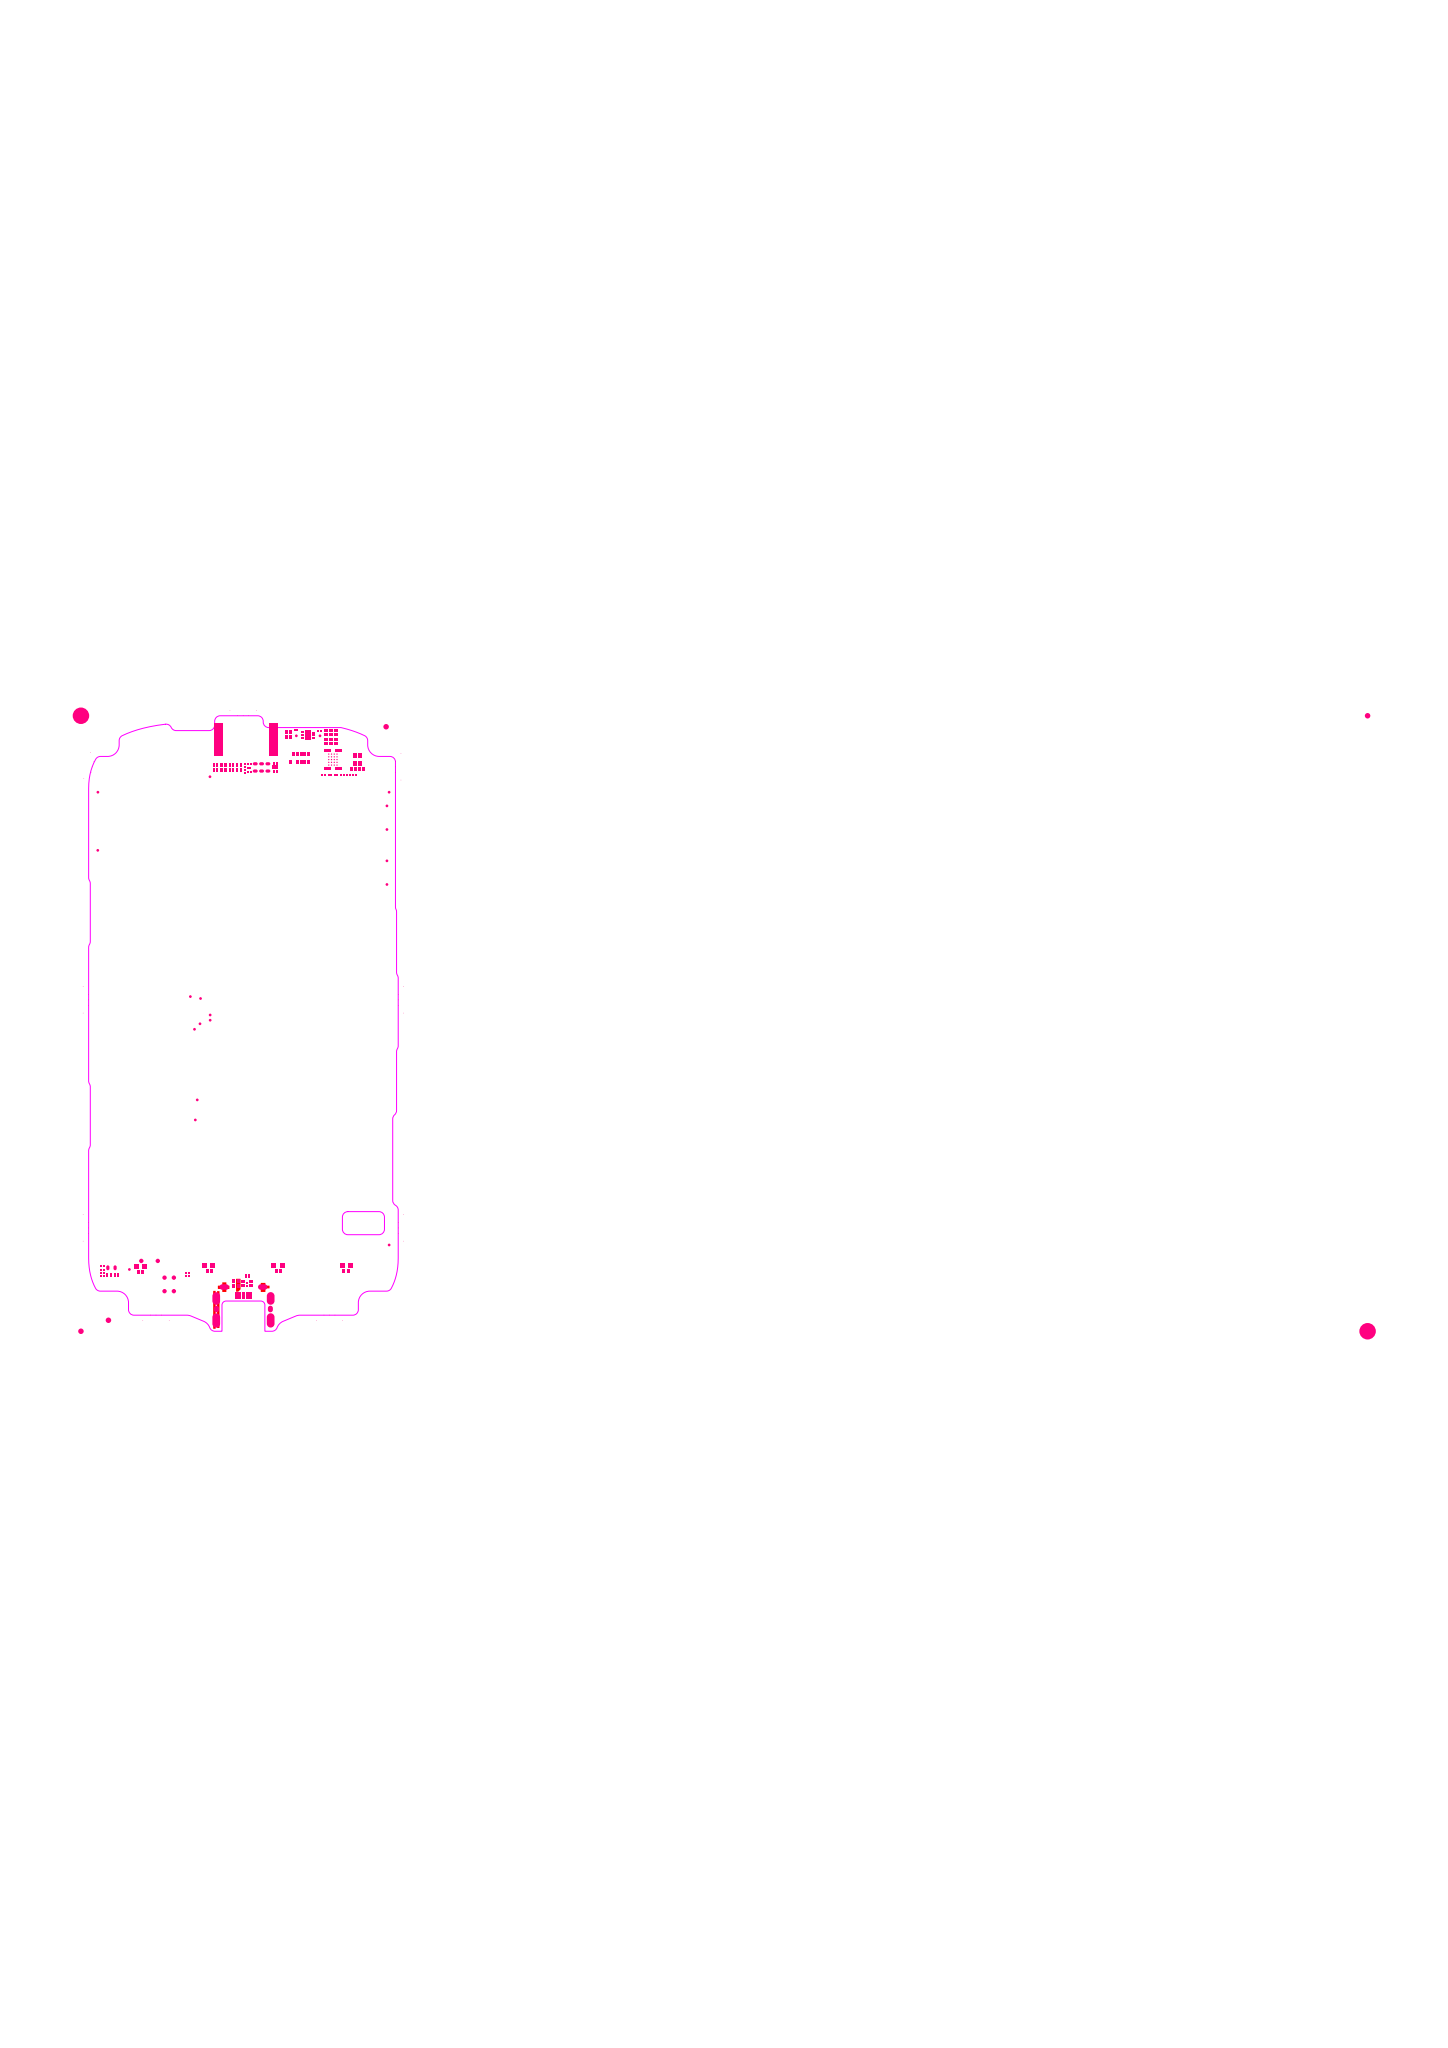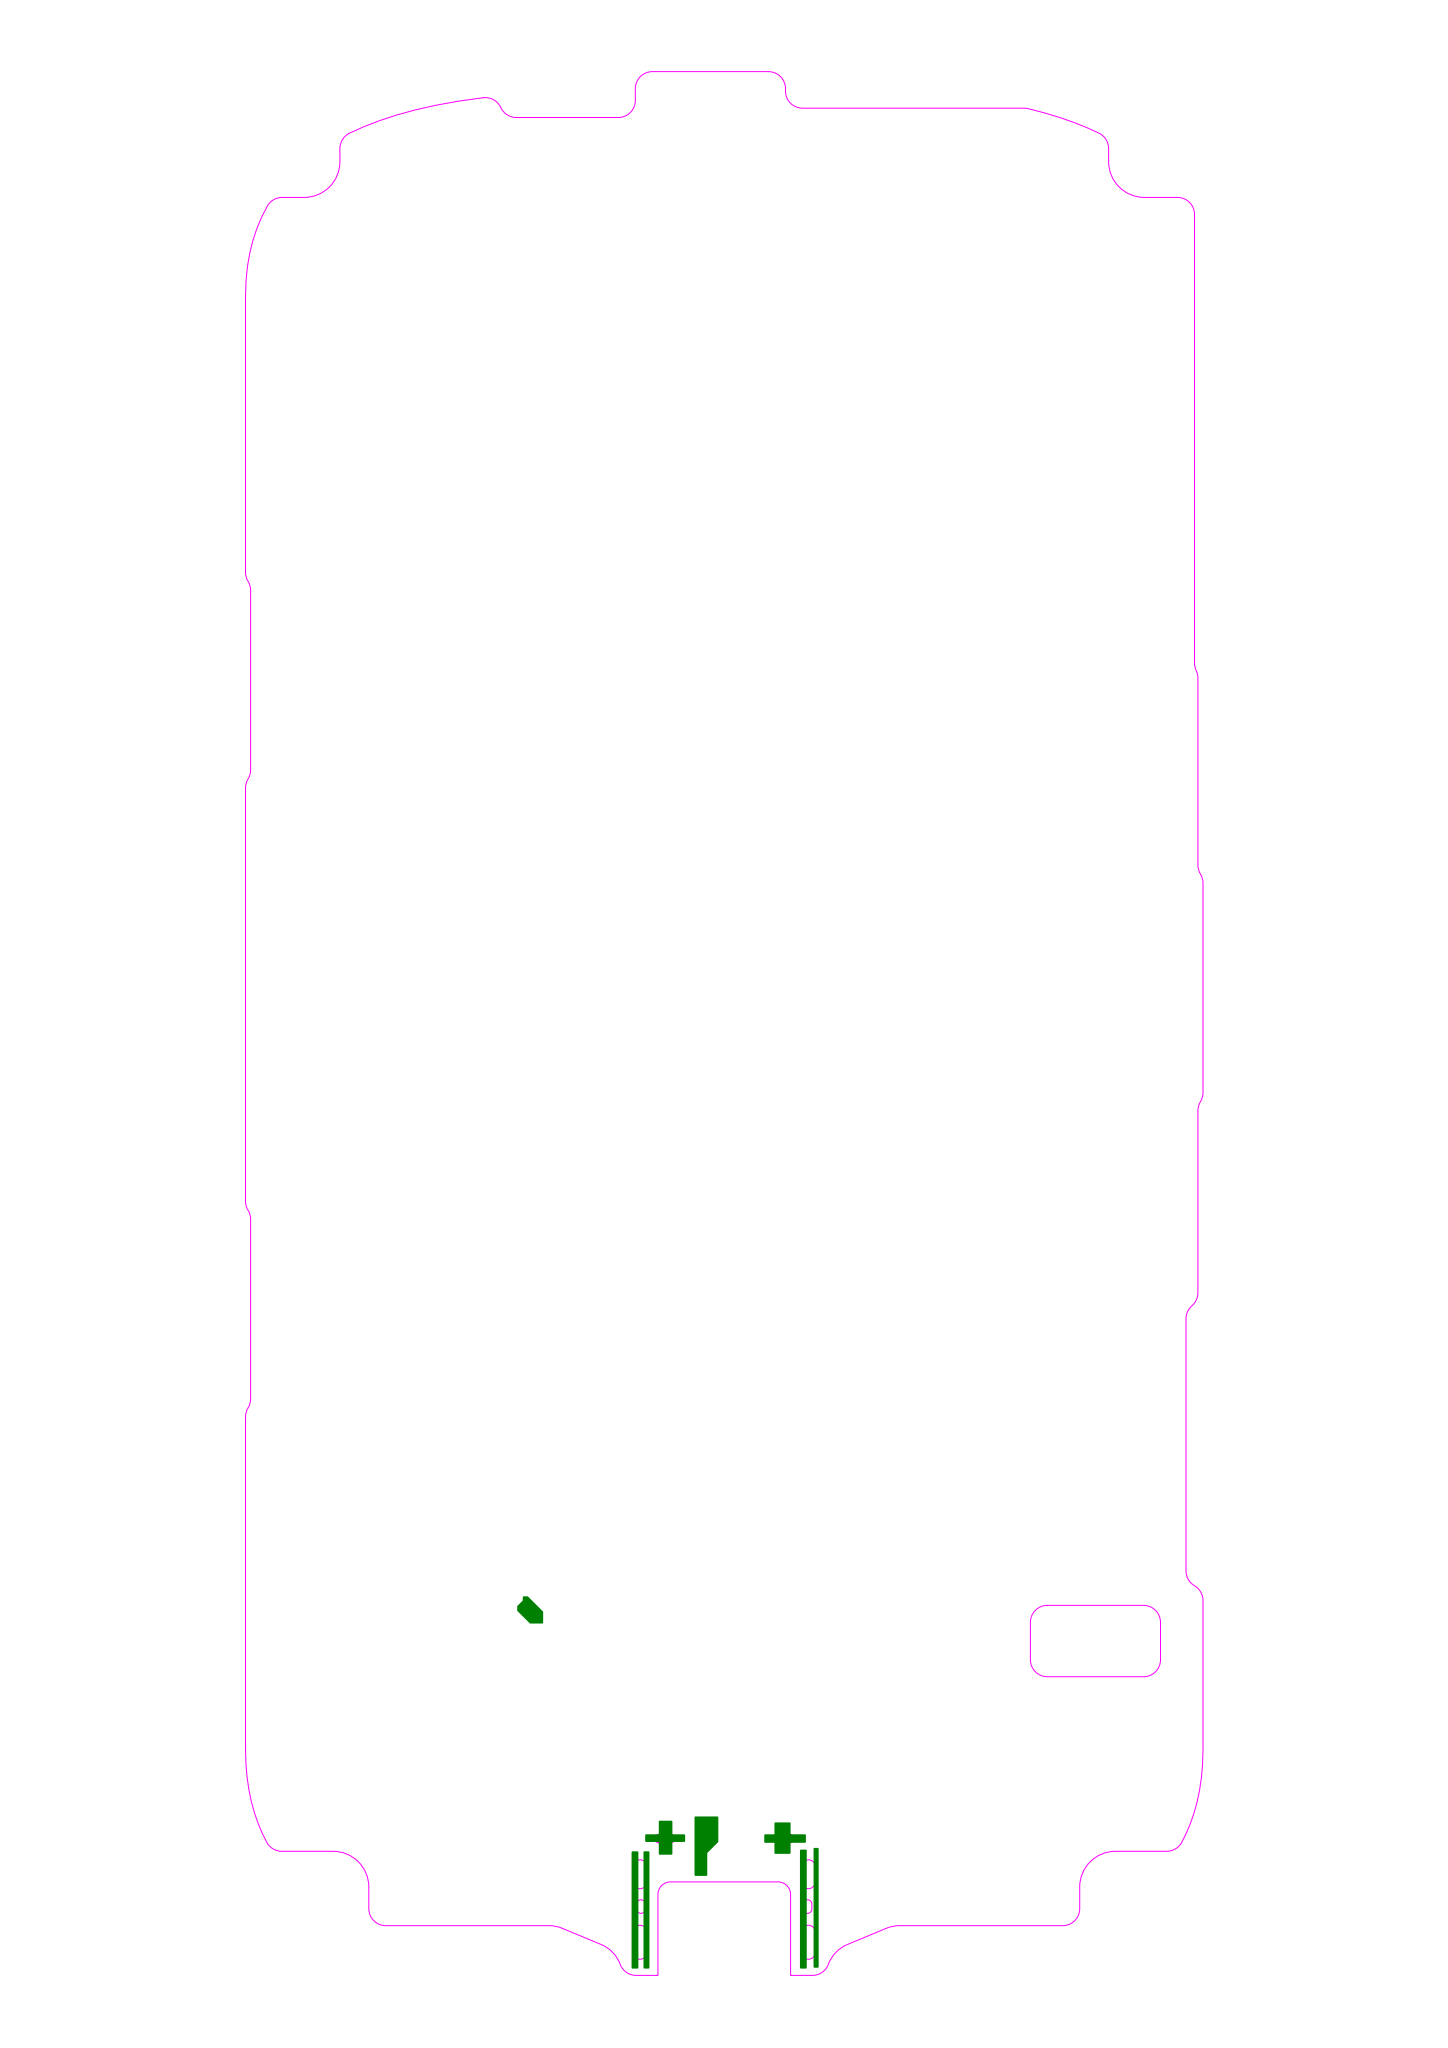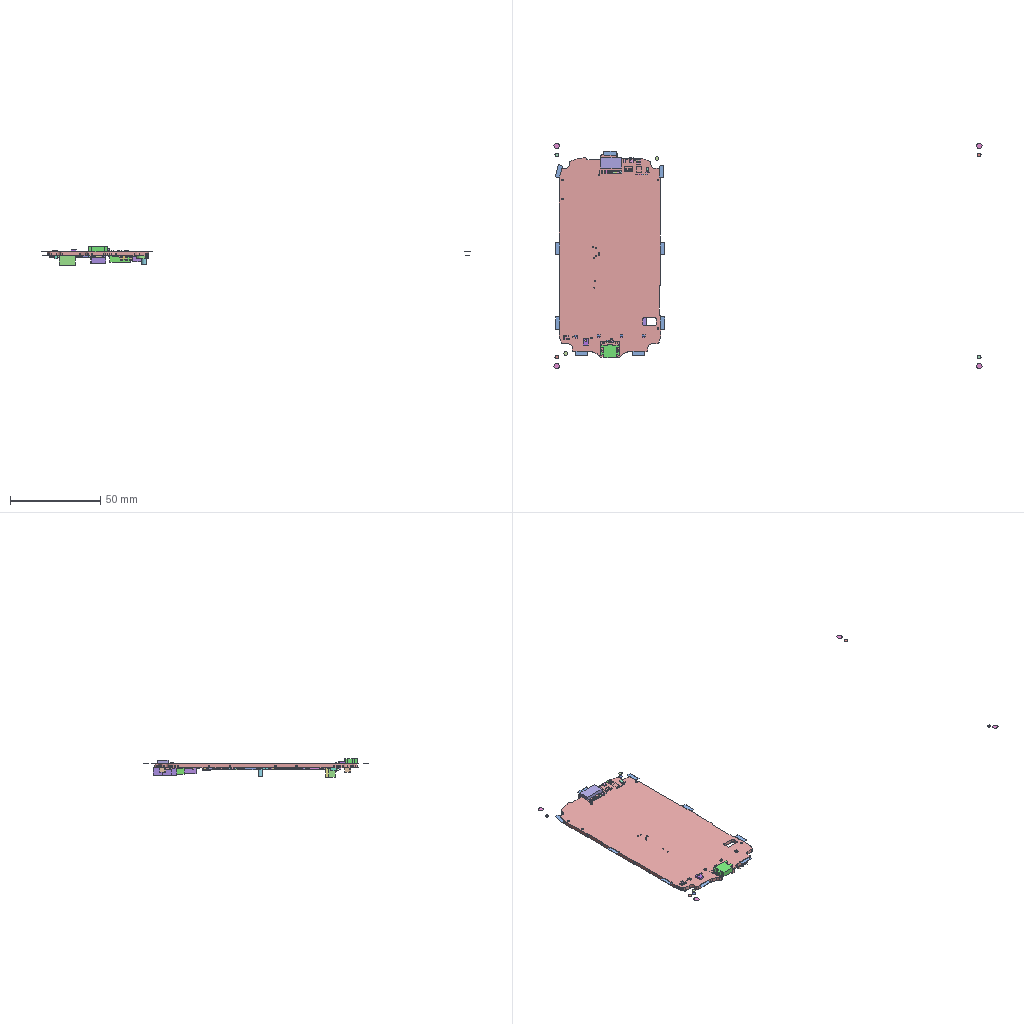Circuit board layout | Siemens PADS | box 237 x 125 x 10.3 mm
Layer stack:
layer,name,type,plane,layer_thickness_mm,copper_thickness_mm,dielectric_constant
0,,,,0,,3.3
1,Top,ROUTING,NONE,0.254,0.03429,4.3
2,Inner Layer 2,ROUTING,NONE,0.254,0.03429,4.3
3,Inner Layer 3,ROUTING,NONE,0.254,0.03429,4.3
4,Inner Layer 4,ROUTING,NONE,0.254,0.03429,4.3
5,Inner Layer 5,ROUTING,NONE,0.254,0.03429,4.3
6,Inner Layer 6,ROUTING,NONE,0.254,0.03429,4.3
7,Inner Layer 7,ROUTING,NONE,0.254,0.03429,4.3
8,Bottom,ROUTING,NONE,0,0.03429,3.3
Part placement, first 418 of 814 lines:
Ref,PartType,Decal,X_mm,Y_mm,Rotation,Layer,Placed,Installed
ANT_GPS1,HT11.011.30120,HT11.011.30120,50.55,117.8,90,Bottom,True,True
ANT_GPS2,HT11.011.30120,HT11.011.30120,53.25,117.8,90,Bottom,True,True
ANT_MAIN1,HT11.011.30120,HT11.011.30120,50.075,15.825,90,Bottom,True,True
ANT_MAIN2,HT11.011.30120,HT11.011.30120,52.775,15.825,90,Bottom,True,True
ANT_MAIN3,HT11.011.30120,HT11.011.30120,47.375,15.825,90,Bottom,True,True
ANT_WLAN1,HT11.011.30120,HT11.011.30120,18.056,118.25,90,Bottom,True,True
ANT_WLAN2,HT11.011.30120,HT11.011.30120,15.35,118.25,90,Bottom,False,True
B201,4700043A001,GZ1005,25.5,60.6,0,Bottom,True,True
B501,4700043A001,GZ1005,25.65,93.05,90,Bottom,True,True
B502,4700043A001,GZ1005,25.65,94.55,90,Bottom,True,True
B503,4700043A001,GZ1005,11.65,103.5,0,Bottom,True,True
B504,4700043A001,GZ1005,11.7,102.45,0,Bottom,True,True
B505,2400006A033,IND0402_0.55,30.9,112.15,180,Top,True,True
B506,2400006A033,IND0402_0.55,30.9,113.1,180,Top,True,True
B507,4700043A001,GZ1005,40.69,114.32,90,Bottom,True,True
B508,4700050A001,GZ1005,41.04,117.62,0,Bottom,True,True
B601,4700039A001,PZ2012U,12.75,29.2,0,Bottom,True,True
B701,4700039A001,PZ2012U,32.5,27.1,270,Bottom,True,True
B901,4700043A001,GZ1005,13,69.05,180,Bottom,True,True
B1001,4700043A001,GZ1005,22,109.9,0,Bottom,True,True
B1101,4700043A001,GZ1005,49.5,118.9,270,Top,True,True
BAT301,KS414F-ER,KS414F-ER,58.15,22.8,90,Bottom,True,True
BREAK1,BREAKAWAY_3,BREAKAWAY_3,6.4,28.8,90,Top,False,True
BREAK2,BREAKAWAY_3,BREAKAWAY_3,18.65,12.95,180,Top,False,True
BREAK3,BREAKAWAY_3,BREAKAWAY_3,50.2,12.95,180,Top,False,True
BREAK5,BREAKAWAY_3,BREAKAWAY_3,34.5,122,0,Top,False,True
BREAK7,BREAKAWAY_3,BREAKAWAY_3,62.7,70.3,270,Top,False,True
BREAK8,BREAKAWAY_3,BREAKAWAY_3,7.1,112.7,75.343,Top,False,True
BREAK9,BREAKAWAY_3,BREAKAWAY_3,6.4,70.3,90,Top,False,True
BREAK10,BREAKAWAY_3,BREAKAWAY_3,62.2,112.7,270,Top,False,True
BREAK11,BREAKAWAY_3,BREAKAWAY_3,62.7,28.8,270,Top,False,True
C101,2100011A026,CAP0603_0.95,34.05,70.95,270,Bottom,True,True
C102,2100015A028,CAP0805_0.95,29.45,60.1,0,Bottom,True,True
C103,2100002A032,CAP0201_0.33,34.4,73.5,270,Bottom,True,True
C104,2100002A021,CAP0201_0.33,20.7,72.9,270,Bottom,True,True
C105,2100002A032,CAP0201_0.33,29.3,61.5,0,Bottom,True,True
C106,2100002A021,CAP0201_0.33,18.1,62.35,270,Bottom,True,True
C107,2100002A032,CAP0201_0.33,20.65,75.15,0,Bottom,True,True
C108,2100002A021_DNP,CAP0201_0.33_DNP,29.3,62.7,0,Bottom,True,True
C109,2100002A032_DNP,CAP0201_0.33_DNP,18.7,62.35,270,Bottom,True,True
C110,2100002A021_DNP,CAP0201_0.33_DNP,18.3,63.45,90,Bottom,True,True
C111,2100002A032_DNP,CAP0201_0.33_DNP,19.9,62.35,270,Bottom,True,True
C112,2100002A021_DNP,CAP0201_0.33_DNP,18.95,63.45,90,Bottom,True,True
C113,2100002A032_DNP,CAP0201_0.33_DNP,20.65,75.75,0,Bottom,True,True
C114,2100002A032,CAP0201_0.33,33.8,73.5,270,Bottom,True,True
C115,2100002A032,CAP0201_0.33,19.6,63.45,90,Bottom,True,True
C116,2100002A032,CAP0201_0.33,20.65,73.95,0,Bottom,True,True
C117,2100002A032,CAP0201_0.33,29.3,62.1,0,Bottom,True,True
C118,2100002A032,CAP0201_0.33,19.3,62.35,270,Bottom,True,True
C119,2100002A032,CAP0201_0.33,35,73,270,Bottom,True,True
C122,2100002A032_DNP,CAP0201_0.33_DNP,20.65,74.55,0,Bottom,True,True
C126,2100015A028,CAP0805_0.95,19.55,64.85,0,Bottom,True,True
C127,2100002A021,CAP0201_0.33,20.5,65.95,180,Bottom,True,True
C128,2100002A032,CAP0201_0.33,19.6,66.2,90,Bottom,True,True
C129,2100002A032_DNP,CAP0201_0.33_DNP,19,66.2,90,Bottom,True,True
C130,2100011A026,CAP0603_0.95,33.3,76.55,90,Bottom,True,True
C131,2100002A021,CAP0201_0.33,33.975,74.95,0,Bottom,True,True
C132,2100002A032,CAP0201_0.33,34.95,81.5,90,Bottom,True,True
C134,2100002A032,CAP0201_0.33,34.95,80.4,270,Bottom,True,True
C137,2100002A032,CAP0201_0.33,34.95,79.3,90,Bottom,True,True
C138,2100002A038,CAP0201_0.33,34.95,78.2,270,Bottom,True,True
C140,2100011A026,CAP0603_0.95,17.4,64.75,270,Bottom,True,True
C141,2100002A038,CAP0201_0.33,18.1,67.4,0,Bottom,True,True
C142,2100002A032,CAP0201_0.33,19,67.3,270,Bottom,True,True
C143,2100002A038,CAP0201_0.33,18.1,66.15,0,Bottom,True,True
C144,2100002A032_DNP,CAP0201_0.33_DNP,19.6,67.3,270,Bottom,True,True
C145,2100002A032_DNP,CAP0201_0.33_DNP,20.2,67.3,270,Bottom,True,True
C146,2100002A032_DNP,CAP0201_0.33_DNP,18.1,66.75,0,Bottom,True,True
C147,2100002A038,CAP0201_0.33,25.65,59.6,270,Bottom,True,True
C148,2100002A038,CAP0201_0.33,26.55,60.6,270,Bottom,True,True
C149,2100002A038,CAP0201_0.33,23.5,61.55,0,Bottom,True,True
C150,2100006A034,CAP0402_0.55,19.9,70.9,0,Bottom,True,True
C151,2100002A038,CAP0201_0.33,20.1,71.7,0,Bottom,True,True
C152,2100002A038,CAP0201_0.33,25.7,62.15,0,Bottom,True,True
C153,2100002A038,CAP0201_0.33,24.6,62.75,180,Bottom,True,True
C154,2100002A038,CAP0201_0.33,25.7,61.55,0,Bottom,True,True
C155,2100002A032_DNP,CAP0201_0.33_DNP,25.7,62.75,0,Bottom,True,True
C156,2100002A032_DNP,CAP0201_0.33_DNP,26.8,61.65,180,Bottom,True,True
C157,2100002A038,CAP0201_0.33,24.6,62.15,180,Bottom,True,True
C158,2100002A038,CAP0201_0.33,23.5,62.75,0,Bottom,True,True
C159,2100002A032_DNP,CAP0201_0.33_DNP,24.6,61.55,180,Bottom,True,True
C160,2100002A038,CAP0201_0.33,16.5,64.6,270,Bottom,True,True
C161,2100002A032_DNP,CAP0201_0.33_DNP,16.25,65.55,0,Bottom,True,True
C162,2100002A038,CAP0201_0.33,34.1,68.9,90,Bottom,True,True
C163,2100002A038,CAP0201_0.33,34.7,68.9,90,Bottom,True,True
C164,2100002A038,CAP0201_0.33,32.5,61.95,270,Bottom,True,True
C165,2100002A038,CAP0201_0.33,35,70.7,270,Bottom,True,True
C166,2100002A038,CAP0201_0.33,23.5,62.15,0,Bottom,True,True
C167,2100002A038,CAP0201_0.33,20.65,76.35,0,Bottom,True,True
C168,2100002A038,CAP0201_0.33,27.4,61.1,0,Bottom,True,True
C173,2100001A024,CAP0201_0.33,11.9,40.55,0,Bottom,True,True
C174,2100002A038,CAP0201_0.33,35.05,74.1,270,Bottom,True,True
C175,2100005A071,CAP0402_0.55,23.5,92.8,180,Bottom,True,True
C176,2100005A071,CAP0402_0.55,23.8,94.1,90,Bottom,True,True
C177,2100002A038,CAP0201_0.33,34.2,76,270,Bottom,True,True
C201,2100001A026,CAP0201_0.33,17.25,62.35,0,Bottom,True,True
C202,2100002A024,CAP0201_0.33,26.55,62.5,270,Bottom,True,True
C203,2100006A050,CAP0402_0.55,28.3,62.1,270,Bottom,True,True
C205,2100001A024,CAP0201_0.33,17.5,59.35,180,Bottom,True,True
C206,2100002A038,CAP0201_0.33,14.15,60.575,90,Bottom,True,True
C207,2100002A036,CAP0201_0.33,17.5,59.95,180,Bottom,True,True
C208,2100001A030,CAP0201_0.33,23.3,58.55,180,Bottom,True,True
C209,2100002A038,CAP0201_0.33,25.65,58.5,90,Bottom,True,True
C214,2100010A076,CAP0603_0.9,34.7,65.45,270,Bottom,True,True
C219,2100006A050,CAP0402_0.55,12.85,60,270,Bottom,True,True
C301,2100006A034,CAP0402_0.55,60.55,27,180,Bottom,True,True
C302,2100001A019,CAP0201_0.33,25.1,45.4,90,Bottom,True,True
C303,2100001A019,CAP0201_0.33,25.1,44.2,90,Bottom,True,True
C304,2100001A024_DNP,CAP0201_0.33_DNP,30.75,45.675,0,Bottom,True,True
C305,2100001A030,CAP0201_0.33,20.2,54.05,180,Bottom,True,True
C306,2100015A028,CAP0805_0.95,33.6,56.25,180,Bottom,True,True
C307,2100002A038,CAP0201_0.33,33.35,48.25,180,Bottom,True,True
C308,2100002A038,CAP0201_0.33,33.35,47.65,180,Bottom,True,True
C309,2100002A038,CAP0201_0.33,31.15,56.9,90,Bottom,True,True
C310,2100011A026,CAP0603_0.95,35.05,48.85,180,Bottom,True,True
C311,2100002A021,CAP0201_0.33,32.5,47.5,90,Bottom,True,True
C312,2100011A026,CAP0603_0.95,35.05,47.65,180,Bottom,True,True
C313,2100002A021,CAP0201_0.33,32.5,46.4,270,Bottom,True,True
C315,2100002A038,CAP0201_0.33,27.9,45.3,90,Bottom,True,True
C316,2100002A038,CAP0201_0.33,33.15,49.7,90,Bottom,True,True
C317,2100002A038,CAP0201_0.33,32.55,49.7,90,Bottom,True,True
C318,2100002A038,CAP0201_0.33,31.75,56.9,90,Bottom,True,True
C319,2100002A038,CAP0201_0.33,23.2,51.7,180,Bottom,True,True
C320,2100002A038,CAP0201_0.33,24.55,53.8,270,Bottom,True,True
C321,2100002A038,CAP0201_0.33,27.9,44.2,270,Bottom,True,True
C322,2100002A038,CAP0201_0.33,33.35,47.05,180,Bottom,True,True
C323,2100002A038,CAP0201_0.33,33.35,48.85,0,Bottom,True,True
C324,2100002A038,CAP0201_0.33,32.55,48.6,90,Bottom,True,True
C325,2100006A061,CAP0402_0.55,23.8,53.9,270,Bottom,True,True
C326,2100006A061,CAP0402_0.55,24.5,50.6,90,Bottom,True,True
C327,2100010A072,CAP0603_0.9,26,39.95,90,Bottom,True,True
C328,2100010A072,CAP0603_0.9,25.45,54.475,270,Bottom,True,True
C329,2100010A072,CAP0603_0.9,31.45,54.35,270,Bottom,True,True
C330,2100002A038,CAP0201_0.33,23.2,55.6,180,Bottom,True,True
C331,2100015A028,CAP0805_0.95,34.55,46.05,180,Bottom,True,True
C332,2100015A028,CAP0805_0.95,25,38.05,0,Bottom,True,True
C333,2100015A028,CAP0805_0.95,31.7,38.45,270,Bottom,True,True
C334,2100010A076,CAP0603_0.9,26.5,42.95,0,Bottom,True,True
C335,2100010A076,CAP0603_0.9,24.35,56.775,90,Bottom,True,True
C336,2100010A076,CAP0603_0.9,23.8,49.25,0,Bottom,True,True
C338,2100002A021,CAP0201_0.33,31.35,40.55,270,Bottom,True,True
C339,2100002A021,CAP0201_0.33,31.95,40.55,270,Bottom,True,True
C340,2100002A021,CAP0201_0.33,26.3,41.7,270,Bottom,True,True
C353,2100002A038,CAP0201_0.33,25.1,43.1,90,Bottom,True,True
C354,2100006A061,CAP0402_0.55,31,55.9,0,Bottom,True,True
C356,2100010A076,CAP0603_0.9,28.1,58.75,180,Bottom,True,True
C357,2100010A072,CAP0603_0.9,35.05,50.05,180,Bottom,True,True
C358,2100010A072,CAP0603_0.9,25.55,56.8,270,Bottom,True,True
C359,2100010A072,CAP0603_0.9,23.15,57.05,270,Bottom,True,True
C360,2100010A072,CAP0603_0.9,30.25,54.35,270,Bottom,True,True
C361,2100010A072,CAP0603_0.9,26.5,45.25,0,Bottom,True,True
C362,2100010A072,CAP0603_0.9,26.5,44.15,180,Bottom,True,True
C363,2100010A072,CAP0603_0.9,23.8,46.85,0,Bottom,True,True
C364,2100010A072_DNP,CAP0603_0.9_DNP,23.8,48.05,0,Bottom,True,True
C366,2100010A076,CAP0603_0.9,29.95,58.05,90,Bottom,True,True
C367,2100010A076,CAP0603_0.9,23.65,52.55,0,Bottom,True,True
C401,2100002A021,CAP0201_0.33,34.95,88.1,90,Bottom,True,True
C402,2100002A032,CAP0201_0.33,34.95,84.8,90,Bottom,True,True
C403,2100002A021,CAP0201_0.33,34.95,85.9,270,Bottom,True,True
C404,2100002A032,CAP0201_0.33,21.05,81.2,270,Bottom,True,True
C405,2100002A021,CAP0201_0.33,21.05,82.3,90,Bottom,True,True
C406,2100002A032,CAP0201_0.33,34.95,87,270,Bottom,True,True
C412,2100011A026,CAP0603_0.95,32.1,76.55,90,Bottom,True,True
C413,2100002A032,CAP0201_0.33,34.95,83.7,270,Bottom,True,True
C414,2100002A038,CAP0201_0.33,34,74.35,0,Bottom,True,True
C415,2100001A024_DNP,CAP0201_0.33_DNP,43.45,103.85,0,Bottom,True,True
C416,2100001A024_DNP,CAP0201_0.33_DNP,43.45,101.55,0,Bottom,True,True
C417,2100001A024_DNP,CAP0201_0.33_DNP,44.7,101.4,0,Bottom,True,True
C418,2100001A024_DNP,CAP0201_0.33_DNP,48.3,103.55,270,Bottom,True,True
C419,2100001A024_DNP,CAP0201_0.33_DNP,49.55,101.55,180,Bottom,True,True
C420,2100001A024_DNP,CAP0201_0.33_DNP,51.35,103.925,180,Bottom,True,True
C421,2100006A050,CAP0402_0.55,46.1,102.15,0,Bottom,True,True
C422,2100005A071,CAP0402_0.55,47.65,102.15,180,Bottom,True,True
C423,2100010A076,CAP0603_0.9,47.2,101,180,Bottom,True,True
C500,2100002A038,CAP0201_0.33,8.89,21.8,0,Top,True,True
C501,2100001A024_DNP,CAP0201_0.33_DNP,8.87,20.65,180,Top,True,True
C502,2100001A024,CAP0201_0.33,8.89,20.05,0,Top,True,True
C503,2100001A024,CAP0201_0.33,8.89,21.2,180,Top,True,True
C509,2100010A076,CAP0603_0.9,10.55,21.55,180,Top,True,True
C511,2100001A024,CAP0201_0.33,35.6,111.85,180,Top,True,True
C512,2100002A001,CAP0201_0.33,35.58,112.57,180,Top,True,True
C513,2100001A024,CAP0201_0.33,35.59,113.23,0,Top,True,True
C514,2100005A071,CAP0402_0.55,14.6,104.1,0,Bottom,True,True
C516,2100005A058_DNP,CAP0402_0.55_DNP,14.25,102.9,270,Bottom,True,True
C517,2100002A038,CAP0201_0.33,29.75,56.05,90,Bottom,True,True
C518,2100002A038,CAP0201_0.33,33.85,64.75,90,Bottom,True,True
C519,2100002A038,CAP0201_0.33,33.85,66,270,Bottom,True,True
C520,2100005A071,CAP0402_0.55,14.6,101.7,180,Bottom,True,True
C521,2100010A076,CAP0603_0.9,28.275,56.025,0,Bottom,True,True
C522,2100002A036,CAP0201_0.33,29.2,53.8,270,Bottom,True,True
C523,2100002A036,CAP0201_0.33,29.2,54.9,90,Bottom,True,True
C524,2100003A017,CAP0201_0.33,19.2,92.85,90,Bottom,True,True
C525,2100003A017,CAP0201_0.33,21,92.85,270,Bottom,True,True
C526,2100015A028,CAP0805_0.95,17.7,94.15,180,Bottom,True,True
C527,2100015A028,CAP0805_0.95,20.9,94.15,0,Bottom,True,True
C530,2100001A024_DNP,CAP0201_0.33_DNP,42.34,113.22,180,Bottom,True,True
C531,2100001A024,CAP0201_0.33,41.14,112.62,180,Bottom,True,True
C533,2100001A024_DNP,CAP0201_0.33_DNP,42.34,111.97,0,Bottom,True,True
C534,2100002A038,CAP0201_0.33,42.34,112.62,0,Bottom,True,True
C535,2100002A038,CAP0201_0.33,41.14,111.97,0,Bottom,True,True
C536,2100010A076,CAP0603_0.9,16.9,85.45,0,Bottom,True,True
C538,2100002A038,CAP0201_0.33,26.55,53.6,0,Bottom,True,True
C539,2100006A061,CAP0402_0.55,26.6,56.15,90,Bottom,True,True
C543,2100001A022,CAP0201_0.33,15.15,44.6,90,Bottom,True,True
C544,2100001A022,CAP0201_0.33,15.75,43.5,90,Bottom,True,True
C545,2100001A022,CAP0201_0.33,15.15,43.5,90,Bottom,True,True
C563,2100002A001,CAP0201_0.33,24.65,20.35,270,Top,True,True
C564,2100001A024,CAP0201_0.33,24.02,20.37,270,Top,True,True
C610,2100005A079_DNP,CAP0402_0.55_DNP,52.3,20.45,180,Bottom,True,True
C611,2100005A079_DNP,CAP0402_0.55_DNP,51.95,23.15,90,Bottom,True,True
C612,2100005A071,CAP0402_0.55,16.3,35.85,180,Bottom,True,True
C618,2400002A008,IND0402_0.55,13.9,37.05,0,Bottom,True,True
C619,2100005A062,CAP0402_0.55,13.75,30.4,180,Bottom,True,True
C620,2100015A028,CAP0805_0.95,16.2,29.1,180,Bottom,True,True
C621,2100005A027,CAP0402_0.55,11.1,37.65,270,Bottom,True,True
C622,2100005A071,CAP0402_0.55,12.25,30.4,0,Bottom,True,True
C623,2100005A005,CAP0402_0.55,15.1,36.55,270,Bottom,True,True
C625,2400002A072,IND0402_0.65,9.85,38,0,Bottom,True,True
C626,2100005A002,CAP0402_0.55,9.85,37.1,180,Bottom,True,True
C628,2100002A021,CAP0201_0.33,19.55,41.05,0,Bottom,True,True
C634,2100002A021,CAP0201_0.33,15.05,30.25,180,Bottom,True,True
C638,2100002A021,CAP0201_0.33,15.05,30.85,180,Bottom,True,True
C640,2100001A025,CAP0201_0.33,10.95,30.55,0,Bottom,True,True
C700,2100005A071,CAP0402_0.55,17.65,35,180,Bottom,True,True
C701,0600003A001,RES0402,24.1,33.8,270,Bottom,True,True
C702,2100001A022,CAP0201_0.33,29.2,29.85,180,Bottom,True,True
C703,2100001A022,CAP0201_0.33,29.15,29.2,0,Bottom,True,True
C704,2100001A030,CAP0201_0.33,30.4,29.95,0,Bottom,True,True
C705,2100006A023,CAP0402_0.55,32.75,30.6,270,Bottom,True,True
C706,2100006A050,CAP0402_0.55,32.75,32.1,90,Bottom,True,True
C707,2100011A026,CAP0603_0.95,32.1,29.25,0,Bottom,True,True
C708,2100001A030,CAP0201_0.33,23.5,30.35,0,Bottom,True,True
C718,2100001A022,CAP0201_0.33,21.2,28.65,0,Bottom,True,True
C719,2100001A022,CAP0201_0.33,20.1,28.65,0,Bottom,True,True
C720,2100001A030,CAP0201_0.33,22.3,28.65,180,Bottom,True,True
C721,2100006A010,CAP0402_0.55,21.5,32.85,180,Bottom,True,True
C722,2100010A076,CAP0603_0.9,19.5,33.3,41.186,Bottom,True,True
C724,2100005A079_DNP,CAP0402_0.55_DNP,18.85,30.85,270,Bottom,True,True
C725,2100005A079,CAP0402_0.55,17.25,30.95,0,Bottom,True,True
C726,2400002A017,IND0402_0.55,30,26.2,0,Bottom,True,True
C727,2100001A022,CAP0201_0.33,29.8,25.45,180,Bottom,True,True
C728,2100001A022,CAP0201_0.33,29.8,24.85,180,Bottom,True,True
C729,2100001A030,CAP0201_0.33,29.8,24.25,180,Bottom,True,True
C730,2100006A010,CAP0402_0.55,28.8,27.85,90,Bottom,True,True
C731,2100010A076,CAP0603_0.9,30.35,28.4,90,Bottom,True,True
C732,2100001A015,CAP0201_0.33,25.45,26.45,90,Bottom,True,True
C735,2100001A004_DNP,CAP0201_0.33_DNP,25.4,25.35,270,Bottom,True,True
C736,2100001A004_DNP,CAP0201_0.33_DNP,25.85,27.3,180,Bottom,True,True
C737,0600003A001,RES0402,23.2,33.35,90,Bottom,True,True
C738,2400002A016_DNP,IND0402_0.55_DNP,23.675,31.8,0,Bottom,True,True
C800,2100002A038,CAP0201_0.33,10.475,55.4,90,Bottom,True,True
C806,2100001A030,CAP0201_0.33,8.6,54.85,0,Bottom,True,True
C807,2100002A038,CAP0201_0.33,8.6,55.55,0,Bottom,True,True
C809,2100001A030,CAP0201_0.33,18,41.8,270,Bottom,True,True
C810,2100001A030,CAP0201_0.33,8.7,48.15,180,Bottom,True,True
C811,2100001A022,CAP0201_0.33,8.725,47.55,180,Bottom,True,True
C812,2100002A001,CAP0201_0.33,14.1,40.55,0,Bottom,True,True
C813,2100001A004_DNP,CAP0201_0.33_DNP,12.4,43.15,0,Bottom,True,True
C814,2100001A022,CAP0201_0.33,15.75,44.6,90,Bottom,True,True
C815,2100001A004_DNP,CAP0201_0.33_DNP,10.925,43.125,0,Bottom,True,True
C817,2100001A022,CAP0201_0.33,17.2,44.65,180,Bottom,True,True
C818,2100002A021,CAP0201_0.33,13.85,54.8,90,Bottom,True,True
C819,2100002A014,CAP0201_0.33,8.6,51.85,0,Bottom,True,True
C820,2100002A032,CAP0201_0.33,20.1,52.05,180,Bottom,True,True
C821,2100006A050_DNP,CAP0402_0.55_DNP,8.8,54,0,Bottom,True,True
C822,2100001A030,CAP0201_0.33,13,54.45,180,Bottom,True,True
C823,2100001A004,CAP0201_0.33,8.7,49.95,0,Bottom,True,True
C824,2400001A008,IND0201_0.33,8.7,48.75,180,Bottom,True,True
C825,2100002A014,CAP0201_0.33,8.55,52.45,0,Bottom,True,True
C827,2100001A024,CAP0201_0.33,8.6,43.95,0,Bottom,True,True
C828,2100001A011,CAP0201_0.33,8.6,45.15,0,Bottom,True,True
C829,2100001A004,CAP0201_0.33,19.7,45.3,0,Bottom,True,True
C830,2100001A022,CAP0201_0.33,11.3,55.05,0,Bottom,True,True
C831,2100002A038,CAP0201_0.33,14.05,55.65,180,Bottom,True,True
C832,2100010A076,CAP0603_0.9,14.25,56.55,180,Bottom,True,True
C833,2100010A076,CAP0603_0.9,19.55,50.55,180,Bottom,True,True
C834,2100002A021,CAP0201_0.33,12.4,55.65,180,Bottom,True,True
C835,2100001A004,CAP0201_0.33,19.7,44.7,0,Bottom,True,True
C836,2100011A026,CAP0603_0.95,9.15,56.55,0,Bottom,True,True
C837,2100010A076,CAP0603_0.9,19.55,52.95,180,Bottom,True,True
C839,2100001A030,CAP0201_0.33,17.35,41.8,270,Bottom,True,True
C842,2100002A038,CAP0201_0.33,11.3,54.45,0,Bottom,True,True
C847,2100001A022,CAP0201_0.33,12.85,56.5,90,Bottom,True,True
C848,2100001A001_DNP,CAP0201_0.33_DNP,13.65,43.15,0,Bottom,True,True
C849,2100002A001,CAP0201_0.33,15.2,40.75,0,Bottom,True,True
C850,2100001A024,CAP0201_0.33,9.7,40.55,0,Bottom,True,True
C851,2100002A038,CAP0201_0.33,19,51.45,180,Bottom,True,True
C854,2100001A024,CAP0201_0.33,44.05,112.55,270,Bottom,True,True
C855,2100005A087,CAP0402_0.55,42.59,117.82,90,Bottom,True,True
C856,2100006A050,CAP0402_0.55,42.84,116.52,0,Bottom,True,True
C857,2100005A074,CAP0402_0.55,42.84,113.97,0,Bottom,True,True
C859,2100005A008_DNP,CAP0402_0.55_DNP,53.7,112.1,180,Bottom,True,True
C860,0600003A001,RES0402,53.35,113.25,90,Bottom,True,True
C861,2100002A014,CAP0201_0.33,8.6,51.2,0,Bottom,True,True
C862,2100005A008_DNP,CAP0402_0.55_DNP,53,114.45,0,Bottom,True,True
C863,2100002A032,CAP0201_0.33,16,56.25,0,Bottom,True,True
C864,2100002A014,CAP0201_0.33,8.6,53.05,0,Bottom,True,True
C865,2100002A021,CAP0201_0.33,15.05,55.4,270,Bottom,True,True
C866,2100002A038,CAP0201_0.33,13,55.05,180,Bottom,True,True
C869,2100002A038,CAP0201_0.33,16.25,55.4,270,Bottom,True,True
C870,2100001A022,CAP0201_0.33,19,52.05,180,Bottom,True,True
C871,2100001A004_DNP,CAP0201_0.33_DNP,9.55,43.075,0,Bottom,True,True
C872,2100001A024,CAP0201_0.33,15.65,55.4,270,Bottom,True,True
C873,2100001A004,CAP0201_0.33,19.8,46.5,0,Bottom,True,True
C874,2100002A038,CAP0201_0.33,17.5,42.75,180,Bottom,True,True
C875,2100001A004,CAP0201_0.33,19.8,45.9,0,Bottom,True,True
C876,2100001A024,CAP0201_0.33,18.8,49.65,0,Bottom,True,True
C877,2100001A024,CAP0201_0.33,18.8,49,0,Bottom,True,True
C878,2100001A030,CAP0201_0.33,8.725,46.95,180,Bottom,True,True
C879,2100002A021,CAP0201_0.33,18,54.05,0,Bottom,True,True
C881,2100002A032,CAP0201_0.33,19.1,54.05,180,Bottom,True,True
C884,2100001A024,CAP0201_0.33,8.725,46.35,0,Bottom,True,True
C888,2100001A024,CAP0201_0.33,8.7,50.55,0,Bottom,True,True
C889,2100001A022_DNP,CAP0201_0.33_DNP,18.2,45,90,Bottom,True,True
C892,2100002A038,CAP0201_0.33,10.2,54.45,0,Bottom,True,True
C893,2100001A024,CAP0201_0.33,16.35,42.9,270,Bottom,True,True
C894,2100001A013,CAP0201_0.33,16.35,44.6,270,Bottom,True,True
C895,2100010A076_DNP,CAP0603_0.9_DNP,11.35,56.55,180,Bottom,True,True
C899,2100002A032,CAP0201_0.33,12.15,54.8,90,Bottom,True,True
C901,2100010A076,CAP0603_0.9,15.7,71.2,0,Bottom,True,True
C902,2100010A076,CAP0603_0.9,17.9,71.25,180,Bottom,True,True
C903,2100002A038,CAP0201_0.33,20.05,77.35,180,Bottom,True,True
C904,2100010A072,CAP0603_0.9,13.2,71.25,180,Bottom,True,True
C905,2100002A038,CAP0201_0.33,14.1,70,270,Bottom,True,True
C906,2100002A038,CAP0201_0.33,14.35,82.55,90,Bottom,True,True
C907,2100002A038,CAP0201_0.33,20.05,80.35,180,Bottom,True,True
C908,2100011A026,CAP0603_0.95,15.45,68.75,180,Bottom,True,True
C909,2100010A076,CAP0603_0.9,10.4,66.375,0,Bottom,True,True
C910,2100011A026,CAP0603_0.95,13.35,67,0,Bottom,True,True
C914,2100011A026,CAP0603_0.95,10.75,71.25,0,Bottom,True,True
C915,2100002A038,CAP0201_0.33,19.8,76.5,90,Bottom,True,True
C917,2100005A058_DNP,CAP0402_0.55_DNP,15.7,111.3,180,Bottom,True,True
C918,2100005A058_DNP,CAP0402_0.55_DNP,15.7,113.9,180,Bottom,True,True
C919,2100002A038_DNP,CAP0201_0.33_DNP,19.05,84.55,180,Bottom,True,True
C920,2100005A079,CAP0402_0.55,16.95,82.8,180,Bottom,True,True
C921,2100005A079_DNP,CAP0402_0.55_DNP,15.45,82.35,180,Bottom,True,True
C922,2100005A058_DNP,CAP0402_0.55_DNP,9.1,80.45,90,Bottom,True,True
C923,2100006A023,CAP0402_0.55,9.1,78.95,90,Bottom,True,True
C924,2100005A058_DNP,CAP0402_0.55_DNP,9.1,77.45,270,Bottom,True,True
C928,2100006A061,CAP0402_0.55,33.2,62.35,90,Bottom,True,True
C929,2100006A061,CAP0402_0.55,34.35,63.3,0,Bottom,True,True
C930,2100006A061,CAP0402_0.55,34.5,62.4,0,Bottom,True,True
C931,2100006A061,CAP0402_0.55,34.6,61.45,180,Bottom,True,True
C1001,2100021A086,PCAP3216_1.2,11.35,23.05,270,Bottom,True,True
C1002,2100005A071,CAP0402_0.55,12.1,26,90,Bottom,True,True
C1003,2100006A023,CAP0402_0.55,11.2,26,90,Bottom,True,True
C1005,2100002A032,CAP0201_0.33,23.85,25.45,90,Bottom,True,True
C1006,2100005A071,CAP0402_0.55,59.65,69.45,90,Bottom,True,True
C1007,2100005A071,CAP0402_0.55,60.8,69.45,90,Bottom,True,True
C1008,2100006A050,CAP0402_0.55,60.05,72.625,0,Bottom,True,True
C1009,2100005A071,CAP0402_0.55,61.375,71.2,270,Bottom,True,True
C1010,2100006A050,CAP0402_0.55,59.85,77.05,0,Bottom,True,True
C1011,2100005A071,CAP0402_0.55,33.2,19.2,180,Top,True,True
C1012,2100006A050,CAP0402_0.55,61.35,77.05,180,Bottom,True,True
C1013,2100010A071,CAP0603_0.9,35.45,26,0,Bottom,True,True
C1014,2100010A076,CAP0603_0.9,35.45,29.5,0,Bottom,True,True
C1015,2100005A070,CAP0402_0.55,59.9,111.7,180,Bottom,True,True
C1017,2100010A072,CAP0603_0.9,36.7,112.6,270,Top,True,True
C1019,2100006A061,CAP0402_0.55,22.35,106.75,0,Bottom,True,True
C1020,2100001A014,CAP0201_0.33,35.25,18.55,90,Top,True,True
C1021,2100010A076,CAP0603_0.9,21.4,114.3,90,Bottom,True,True
C1022,2100002A038,CAP0201_0.33,49.1,111.15,0,Top,True,True
C1023,2100010A076,CAP0603_0.9,39,112.6,90,Top,True,True
C1025,2100006A061,CAP0402_0.55,42.7,118.1,180,Top,True,True
C1027,2100006A050,CAP0402_0.55,22.25,107.725,180,Bottom,True,True
C1028,2100005A071,CAP0402_0.55,54.05,26.05,270,Bottom,True,True
C1029,2100001A024,CAP0201_0.33,55.6,27.15,180,Bottom,True,True
C1030,2100006A050,CAP0402_0.55,58.1,27,180,Bottom,True,True
C1031,2100001A024,CAP0201_0.33,56.95,26.25,270,Bottom,True,True
C1033,2100006A050,CAP0402_0.55,60.8,83.95,90,Bottom,True,True
C1034,2100011A026,CAP0603_0.95,59.7,84.3,90,Bottom,True,True
C1101,2100002A038,CAP0201_0.33,52.5,111.15,180,Top,True,True
C1102,2100002A038,CAP0201_0.33,54.7,111.15,0,Top,True,True
C1104,2100006A061,CAP0402_0.55,59.3,53.15,90,Bottom,True,True
C1105,2100006A061,CAP0402_0.55,58.35,53.15,90,Bottom,True,True
C1106,2100006A050,CAP0402_0.55,56.4,53.15,270,Bottom,True,True
C1107,2100005A071_DNP,CAP0402_0.55_DNP,60.4,53.15,90,Bottom,True,True
C1108,2100001A024_DNP,CAP0201_0.33_DNP,26.85,94.7,0,Bottom,True,True
C1109,2100001A024_DNP,CAP0201_0.33_DNP,26.85,92.3,0,Bottom,True,True
C1110,2100006A061,CAP0402_0.55,25.2,91.25,180,Bottom,True,True
C1111,2100001A024_DNP,CAP0201_0.33_DNP,29.25,94.6,0,Bottom,True,True
C1112,2100001A024_DNP,CAP0201_0.33_DNP,26.85,93.5,0,Bottom,True,True
C1113,2100001A024_DNP,CAP0201_0.33_DNP,28.1,94.5,0,Bottom,True,True
C1114,2100001A024_DNP,CAP0201_0.33_DNP,28.2,92.65,270,Bottom,True,True
C1115,2100001A024_DNP,CAP0201_0.33_DNP,29.25,95.2,0,Bottom,True,True
C1116,2100001A024_DNP,CAP0201_0.33_DNP,28.1,95.2,0,Bottom,True,True
C1117,2100001A024_DNP,CAP0201_0.33_DNP,26.85,95.3,0,Bottom,True,True
C1118,2100002A038,CAP0201_0.33,26.9,91.65,0,Bottom,True,True
C1119,2100001A024_DNP,CAP0201_0.33_DNP,29.2,91.9,0,Bottom,True,True
C1120,2100001A024_DNP,CAP0201_0.33_DNP,29.25,92.7,0,Bottom,True,True
C1121,2100001A024_DNP,CAP0201_0.33_DNP,26.85,92.9,180,Bottom,True,True
C1122,2100002A038,CAP0201_0.33,29.25,93.35,0,Bottom,True,True
C1123,2100006A061,CAP0402_0.55,50.4,117.4,270,Top,True,True
C1124,2100002A038,CAP0201_0.33,26.8,90.1,0,Bottom,True,True
C1125,2100002A038,CAP0201_0.33,26.85,94.1,0,Bottom,True,True
C1127,2100006A061,CAP0402_0.55,51.3,118.9,270,Top,True,True
C1128,2100001A024_DNP,CAP0201_0.33_DNP,28.6,90.5,0,Bottom,True,True
C1129,2100006A061,CAP0402_0.55,26.85,90.85,0,Bottom,True,True
C1135,2100006A061,CAP0402_0.55,51.3,117.4,270,Top,True,True
C1142,2100006A061,CAP0402_0.55,50.4,118.9,270,Top,True,True
C1143,2100006A061,CAP0402_0.55,49.5,117.4,270,Top,True,True
C1144,2100006A061,CAP0402_0.55,42.7,119,180,Top,True,True
CN401,WKTFH001-001,WKTFH001-001,46.875,110.05,0,Bottom,True,True
CN501,KJA133BY01R,KJA133BY01R,34.6,115.8,270,Bottom,False,True
CN600,0900547A001,ECT818000001,48.625,22.7,180,Bottom,True,True
CN1001,SIMF006M5K36-00R,SIMF006M5K36-00RA,47.725,76.725,270,Bottom,True,True
CN1002,USBF005G2K33-00R,USBF005G2K33-00R,34.555,16.475,0,Top,False,True
CN1003,BAT30-03V13-TP540,BAT30-03V13-TP540A,17.475,23.6,180,Bottom,True,True
CN1004,SIMF006M5K36-00R,SIMF006M5K36-00R,44.975,36.7,90,Bottom,False,True
CN1005,FH19C-8S-0.5SH(05),FH19C-8S-0.5SH(05),25.325,115.025,180,Bottom,True,True
CN1101,0900053A001,FH26-45S-0.3SHW,57.575,41.2,270,Bottom,True,True
CN1102,DF30FC-24DS-0.4V,DF30FC-24DS-0.4V,34.56,92.925,0,Bottom,True,True
D202,4800071A001,UMD2_0.9,33.5,60.1,0,Bottom,True,True
D203,4800388A001,EMD2_0.7,31,61.45,0,Bottom,True,True
D204,4800071A001,UMD2_0.9,11,61.65,180,Bottom,True,True
D205,4800071A001,UMD2_0.9,10.75,60.05,180,Bottom,True,True
D301,4800071A001,UMD2_0.9,21.55,60.7,90,Bottom,True,True
Pad and via stacks:
via_name,drill_mm,start_layer,end_layer,type,pad_size_top,pad_size_inner,pad_size_bottom
JMPVIA_AAAAA,0.9398,1,8,through,1.397,1.778,1.397
STANDARDVIA,0.9398,1,8,through,1.397,1.397,1.397
Design rules, without the lines most boards share:
# PADS Layout design rules of , as PADS writes them (units: mm)
THERLINEWID 0.381
THERSMDWID 0.254
THERFLAGS 135423
HATCHGRID 0.11
MINHATAREA 0.2
HATCHMODE 0
DRILLHOLE 0.1524
DRLOVERSIZE 0
VIAMODE A
LAYERPAIR 2      7
TEARDROP 2713690
RULES_SECTION METRIC
{
NET_CLASS DATA
GROUP DATA
ASSOCIATED_NET DATA
DESIGN RULES
{
RULE_SET (1)
{
FOR :
{
DEFAULT :
}
AGAINST :
{
DEFAULT :
}
LAYER 0
CLEARANCE_RULE :
{
TRACK_TO_TRACK 0.1524
VIA_TO_TRACK 0.1524
VIA_TO_VIA 0.1524
PAD_TO_TRACK 0.1524
PAD_TO_VIA 0.1524
PAD_TO_PAD 0.1524
SMD_TO_TRACK 0.1524
SMD_TO_VIA 0.1524
SMD_TO_PAD 0.1524
SMD_TO_SMD 0.1524
COPPER_TO_TRACK 0.1524
COPPER_TO_VIA 0.1524
COPPER_TO_PAD 0.1524
COPPER_TO_SMD 0.1524
COPPER_TO_COPPER 0.1524
TEXT_TO_TRACK 0.1524
TEXT_TO_VIA 0.1524
TEXT_TO_PAD 0.1524
TEXT_TO_SMD 0.1524
OUTLINE_TO_TRACK 0.1524
OUTLINE_TO_VIA 0.1524
OUTLINE_TO_PAD 0.1524
OUTLINE_TO_SMD 0.1524
OUTLINE_TO_COPPER 0.1524
DRILL_TO_TRACK 0.1524
DRILL_TO_VIA 0.1524
DRILL_TO_PAD 0.1524
DRILL_TO_SMD 0.1524
DRILL_TO_COPPER 0.1524
SAME_NET_SMD_TO_VIA 0.1524
SAME_NET_SMD_TO_CRN 0.1524
SAME_NET_VIA_TO_VIA 0.1524
SAME_NET_PAD_TO_CRN 0.1524
MIN_TRACK_WIDTH 0.3048
REC_TRACK_WIDTH 0.3048
MAX_TRACK_WIDTH 0.3048
DRILL_TO_DRILL 0.1524
BODY_TO_BODY 0.1524
SAME_NET_TRACK_TO_CRN 0
}
}
RULE_SET (2)
{
FOR :
{
DEFAULT :
}
AGAINST :
{
DEFAULT :
}
LAYER 0
HIGH_SPEED_RULE :
{
MIN_LENGTH 0
MAX_LENGTH 1270
STUB_LENGTH 0
PARALLEL_LENGTH 25.4
PARALLEL_GAP 5.08
TANDEM_LENGTH 25.4
TANDEM_GAP 5.08
MIN_DELAY 0
MAX_DELAY 10
MIN_CAPACITANCE 0
MAX_CAPACITANCE 10
MIN_IMPEDANCE 50
MAX_IMPEDANCE 150
SHIELD_NET *
SHIELD_GAP 5.08
MATCH_LENGTH_TOLERANCE 5.08
}
}
RULE_SET (3)
{
FOR :
{
DEFAULT :
}
AGAINST :
{
DEFAULT :
}
LAYER 0
ROUTE_RULE :
{
LENGTH_MINIMIZATION_TYPE 1
VIA_SHARE Y
TRACE_SHARE Y
AUTO_ROUTE Y
RIPUP Y
SHOVE Y
ROUTE_PRIORITY 3
MAX_NUMBER_OF_VIAS -1
VALID_LAYER 1
VALID_LAYER 2
VALID_VIA_TYPE STANDARDVIA
}
}
}
}
Classes set for this board:
# PADS net classes of 
NET_CLASS DATA
GROUP DATA
ASSOCIATED_NET DATA
DESIGN RULES
{
RULE_SET (1)
{
FOR :
{
DEFAULT :
}
AGAINST :
{
DEFAULT :
}
LAYER 0
CLEARANCE_RULE :
{
TRACK_TO_TRACK 0.1524
VIA_TO_TRACK 0.1524
VIA_TO_VIA 0.1524
PAD_TO_TRACK 0.1524
PAD_TO_VIA 0.1524
PAD_TO_PAD 0.1524
SMD_TO_TRACK 0.1524
SMD_TO_VIA 0.1524
SMD_TO_PAD 0.1524
SMD_TO_SMD 0.1524
COPPER_TO_TRACK 0.1524
COPPER_TO_VIA 0.1524
COPPER_TO_PAD 0.1524
COPPER_TO_SMD 0.1524
COPPER_TO_COPPER 0.1524
TEXT_TO_TRACK 0.1524
TEXT_TO_VIA 0.1524
TEXT_TO_PAD 0.1524
TEXT_TO_SMD 0.1524
OUTLINE_TO_TRACK 0.1524
OUTLINE_TO_VIA 0.1524
OUTLINE_TO_PAD 0.1524
OUTLINE_TO_SMD 0.1524
OUTLINE_TO_COPPER 0.1524
DRILL_TO_TRACK 0.1524
DRILL_TO_VIA 0.1524
DRILL_TO_PAD 0.1524
DRILL_TO_SMD 0.1524
DRILL_TO_COPPER 0.1524
SAME_NET_SMD_TO_VIA 0.1524
SAME_NET_SMD_TO_CRN 0.1524
SAME_NET_VIA_TO_VIA 0.1524
SAME_NET_PAD_TO_CRN 0.1524
MIN_TRACK_WIDTH 0.3048
REC_TRACK_WIDTH 0.3048
MAX_TRACK_WIDTH 0.3048
DRILL_TO_DRILL 0.1524
BODY_TO_BODY 0.1524
SAME_NET_TRACK_TO_CRN 0
}
}
RULE_SET (2)
{
FOR :
{
DEFAULT :
}
AGAINST :
{
DEFAULT :
}
LAYER 0
HIGH_SPEED_RULE :
{
MIN_LENGTH 0
MAX_LENGTH 1270
STUB_LENGTH 0
PARALLEL_LENGTH 25.4
PARALLEL_GAP 5.08
TANDEM_LENGTH 25.4
TANDEM_GAP 5.08
MIN_DELAY 0
MAX_DELAY 10
MIN_CAPACITANCE 0
MAX_CAPACITANCE 10
MIN_IMPEDANCE 50
MAX_IMPEDANCE 150
SHIELD_NET *
SHIELD_GAP 5.08
MATCH_LENGTH_TOLERANCE 5.08
}
}
RULE_SET (3)
{
FOR :
{
DEFAULT :
}
AGAINST :
{
DEFAULT :
}
LAYER 0
ROUTE_RULE :
{
LENGTH_MINIMIZATION_TYPE 1
VIA_SHARE Y
TRACE_SHARE Y
AUTO_ROUTE Y
RIPUP Y
SHOVE Y
ROUTE_PRIORITY 3
MAX_NUMBER_OF_VIAS -1
VALID_LAYER 1
VALID_LAYER 2
VALID_VIA_TYPE STANDARDVIA
}
}
}